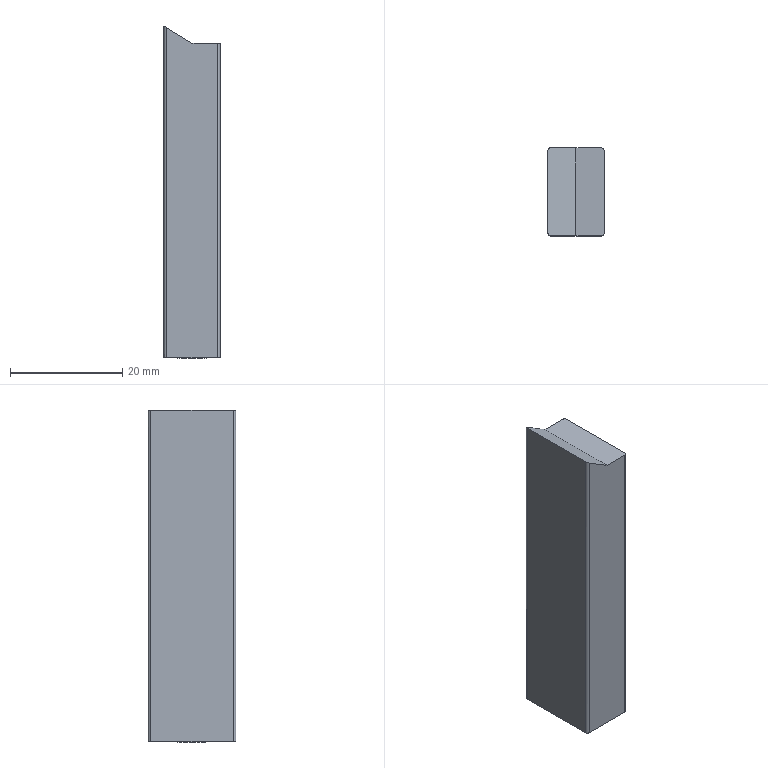Part | STEP file | LUOI GA PHAI TREN | 1 solid | 17 faces | box 10 x 15.6 x 59.05 mm | volume 8567 mm3 | plane 7 | cylinder 6 | cone 4 | commonest cylinder face diameters 1 x4 4.134 x2
STEP:
#1=CARTESIAN_POINT('',(0.,0.,0.));
#2=DIRECTION('',(0.,0.,1.));
#3=DIRECTION('',(1.,0.,0.));
#4=AXIS2_PLACEMENT_3D('',#1,#2,#3);
#5=CARTESIAN_POINT('',(-7.067,7.9,0.5));
#6=VERTEX_POINT('',#5);
#7=CARTESIAN_POINT('',(-7.567,7.9,0.));
#8=VERTEX_POINT('',#7);
#9=CARTESIAN_POINT('',(-7.567,7.9,0.));
#10=DIRECTION('',(-0.7071,0.,-0.7071));
#11=VECTOR('',#10,1.);
#12=LINE('',#9,#11);
#13=CARTESIAN_POINT('',(-5.,7.9,0.));
#14=DIRECTION('',(0.,0.,-1.));
#15=DIRECTION('',(-1.,0.,0.));
#16=AXIS2_PLACEMENT_3D('',#13,#14,#15);
#17=CONICAL_SURFACE('',#16,2.567,0.7854);
#18=CARTESIAN_POINT('',(6.283,0.));
#19=DIRECTION('',(0.,1.));
#20=VECTOR('',#19,1.);
#21=LINE('',#18,#20);
#22=(GEOMETRIC_REPRESENTATION_CONTEXT(2)PARAMETRIC_REPRESENTATION_CONTEXT()REPRESENTATION_CONTEXT('',''));
#23=DEFINITIONAL_REPRESENTATION('',(#21),#22);
#24=PCURVE('',#17,#23);
#25=CARTESIAN_POINT('',(-5.,7.9,0.));
#26=DIRECTION('',(0.,0.,-1.));
#27=DIRECTION('',(-1.,0.,0.));
#28=AXIS2_PLACEMENT_3D('',#25,#26,#27);
#29=CONICAL_SURFACE('',#28,2.567,0.7854);
#30=CARTESIAN_POINT('',(0.,0.));
#31=DIRECTION('',(0.,1.));
#32=VECTOR('',#31,1.);
#33=LINE('',#30,#32);
#34=(GEOMETRIC_REPRESENTATION_CONTEXT(2)PARAMETRIC_REPRESENTATION_CONTEXT()REPRESENTATION_CONTEXT('',''));
#35=DEFINITIONAL_REPRESENTATION('',(#33),#34);
#36=PCURVE('',#29,#35);
#37=SURFACE_CURVE('',#12,(#24,#36),.PCURVE_S1.);
#38=EDGE_CURVE('',#6,#8,#37,.T.);
#39=ORIENTED_EDGE('',*,*,#38,.T.);
#40=CARTESIAN_POINT('',(-2.433,7.9,0.));
#41=VERTEX_POINT('',#40);
#42=CARTESIAN_POINT('',(-5.,7.9,0.));
#43=DIRECTION('',(0.,0.,-1.));
#44=DIRECTION('',(-1.,0.,0.));
#45=AXIS2_PLACEMENT_3D('',#42,#43,#44);
#46=CIRCLE('',#45,2.567);
#47=CARTESIAN_POINT('',(0.,0.));
#48=DIRECTION('',(1.,0.));
#49=VECTOR('',#48,1.);
#50=LINE('',#47,#49);
#51=(GEOMETRIC_REPRESENTATION_CONTEXT(2)PARAMETRIC_REPRESENTATION_CONTEXT()REPRESENTATION_CONTEXT('',''));
#52=DEFINITIONAL_REPRESENTATION('',(#50),#51);
#53=PCURVE('',#17,#52);
#54=CARTESIAN_POINT('',(-5.,7.8,0.));
#55=DIRECTION('',(0.,0.,1.));
#56=DIRECTION('',(1.,0.,0.));
#57=AXIS2_PLACEMENT_3D('',#54,#55,#56);
#58=PLANE('',#57);
#59=CARTESIAN_POINT('',(-2.567,0.1));
#60=CARTESIAN_POINT('',(-2.567,4.546));
#61=CARTESIAN_POINT('',(1.283,2.323));
#62=CARTESIAN_POINT('',(5.134,0.1));
#63=CARTESIAN_POINT('',(1.283,-2.123));
#64=CARTESIAN_POINT('',(-2.567,-4.346));
#65=CARTESIAN_POINT('',(-2.567,0.1));
#66=(BOUNDED_CURVE()B_SPLINE_CURVE(2,(#59,#60,#61,#62,#63,#64,#65),.UNSPECIFIED.,.T.,.F.)B_SPLINE_CURVE_WITH_KNOTS((1,2,2,2,2,1),(-2.094,0.,2.094,4.189,6.283,8.378),.UNSPECIFIED.)CURVE()GEOMETRIC_REPRESENTATION_ITEM()RATIONAL_B_SPLINE_CURVE((1.,0.5,1.,0.5,1.,0.5,1.))REPRESENTATION_ITEM(''));
#67=(GEOMETRIC_REPRESENTATION_CONTEXT(2)PARAMETRIC_REPRESENTATION_CONTEXT()REPRESENTATION_CONTEXT('',''));
#68=DEFINITIONAL_REPRESENTATION('',(#66),#67);
#69=PCURVE('',#58,#68);
#70=SURFACE_CURVE('',#46,(#53,#69),.PCURVE_S1.);
#71=EDGE_CURVE('',#41,#8,#70,.T.);
#72=ORIENTED_EDGE('',*,*,#71,.F.);
#73=CARTESIAN_POINT('',(-2.933,7.9,0.5));
#74=VERTEX_POINT('',#73);
#75=CARTESIAN_POINT('',(-2.433,7.9,0.));
#76=DIRECTION('',(0.7071,0.,-0.7071));
#77=VECTOR('',#76,1.);
#78=LINE('',#75,#77);
#79=CARTESIAN_POINT('',(3.142,0.));
#80=DIRECTION('',(0.,1.));
#81=VECTOR('',#80,1.);
#82=LINE('',#79,#81);
#83=(GEOMETRIC_REPRESENTATION_CONTEXT(2)PARAMETRIC_REPRESENTATION_CONTEXT()REPRESENTATION_CONTEXT('',''));
#84=DEFINITIONAL_REPRESENTATION('',(#82),#83);
#85=PCURVE('',#17,#84);
#86=CARTESIAN_POINT('',(3.142,0.));
#87=DIRECTION('',(0.,1.));
#88=VECTOR('',#87,1.);
#89=LINE('',#86,#88);
#90=(GEOMETRIC_REPRESENTATION_CONTEXT(2)PARAMETRIC_REPRESENTATION_CONTEXT()REPRESENTATION_CONTEXT('',''));
#91=DEFINITIONAL_REPRESENTATION('',(#89),#90);
#92=PCURVE('',#29,#91);
#93=SURFACE_CURVE('',#78,(#85,#92),.PCURVE_S1.);
#94=EDGE_CURVE('',#74,#41,#93,.T.);
#95=ORIENTED_EDGE('',*,*,#94,.F.);
#96=CARTESIAN_POINT('',(-5.,7.9,0.5));
#97=DIRECTION('',(0.,0.,-1.));
#98=DIRECTION('',(1.,0.,0.));
#99=AXIS2_PLACEMENT_3D('',#96,#97,#98);
#100=CIRCLE('',#99,2.067);
#101=CARTESIAN_POINT('',(3.142,-0.5));
#102=DIRECTION('',(1.,0.));
#103=VECTOR('',#102,1.);
#104=LINE('',#101,#103);
#105=(GEOMETRIC_REPRESENTATION_CONTEXT(2)PARAMETRIC_REPRESENTATION_CONTEXT()REPRESENTATION_CONTEXT('',''));
#106=DEFINITIONAL_REPRESENTATION('',(#104),#105);
#107=PCURVE('',#17,#106);
#108=CARTESIAN_POINT('',(-5.,7.9,10.));
#109=DIRECTION('',(0.,0.,-1.));
#110=DIRECTION('',(-1.,0.,0.));
#111=AXIS2_PLACEMENT_3D('',#108,#109,#110);
#112=CYLINDRICAL_SURFACE('',#111,2.067);
#113=CARTESIAN_POINT('',(3.142,9.5));
#114=DIRECTION('',(1.,0.));
#115=VECTOR('',#114,1.);
#116=LINE('',#113,#115);
#117=(GEOMETRIC_REPRESENTATION_CONTEXT(2)PARAMETRIC_REPRESENTATION_CONTEXT()REPRESENTATION_CONTEXT('',''));
#118=DEFINITIONAL_REPRESENTATION('',(#116),#117);
#119=PCURVE('',#112,#118);
#120=SURFACE_CURVE('',#100,(#107,#119),.PCURVE_S1.);
#121=EDGE_CURVE('',#74,#6,#120,.T.);
#122=ORIENTED_EDGE('',*,*,#121,.T.);
#123=EDGE_LOOP('',(#39,#72,#95,#122));
#124=FACE_BOUND('',#123,.F.);
#125=ADVANCED_FACE('',(#124),#17,.F.);
#126=CARTESIAN_POINT('',(-7.067,7.9,20.));
#127=VERTEX_POINT('',#126);
#128=CARTESIAN_POINT('',(-7.067,7.9,10.));
#129=DIRECTION('',(0.,0.,-1.));
#130=VECTOR('',#129,1.);
#131=LINE('',#128,#130);
#132=CARTESIAN_POINT('',(6.283,0.));
#133=DIRECTION('',(0.,1.));
#134=VECTOR('',#133,1.);
#135=LINE('',#132,#134);
#136=(GEOMETRIC_REPRESENTATION_CONTEXT(2)PARAMETRIC_REPRESENTATION_CONTEXT()REPRESENTATION_CONTEXT('',''));
#137=DEFINITIONAL_REPRESENTATION('',(#135),#136);
#138=PCURVE('',#112,#137);
#139=CARTESIAN_POINT('',(-5.,7.9,10.));
#140=DIRECTION('',(0.,0.,-1.));
#141=DIRECTION('',(-1.,0.,0.));
#142=AXIS2_PLACEMENT_3D('',#139,#140,#141);
#143=CYLINDRICAL_SURFACE('',#142,2.067);
#144=CARTESIAN_POINT('',(0.,0.));
#145=DIRECTION('',(0.,1.));
#146=VECTOR('',#145,1.);
#147=LINE('',#144,#146);
#148=(GEOMETRIC_REPRESENTATION_CONTEXT(2)PARAMETRIC_REPRESENTATION_CONTEXT()REPRESENTATION_CONTEXT('',''));
#149=DEFINITIONAL_REPRESENTATION('',(#147),#148);
#150=PCURVE('',#143,#149);
#151=SURFACE_CURVE('',#131,(#138,#150),.PCURVE_S1.);
#152=EDGE_CURVE('',#127,#6,#151,.T.);
#153=ORIENTED_EDGE('',*,*,#152,.T.);
#154=ORIENTED_EDGE('',*,*,#121,.F.);
#155=CARTESIAN_POINT('',(-2.933,7.9,20.));
#156=VERTEX_POINT('',#155);
#157=CARTESIAN_POINT('',(-2.933,7.9,10.));
#158=DIRECTION('',(0.,0.,-1.));
#159=VECTOR('',#158,1.);
#160=LINE('',#157,#159);
#161=CARTESIAN_POINT('',(3.142,0.));
#162=DIRECTION('',(0.,1.));
#163=VECTOR('',#162,1.);
#164=LINE('',#161,#163);
#165=(GEOMETRIC_REPRESENTATION_CONTEXT(2)PARAMETRIC_REPRESENTATION_CONTEXT()REPRESENTATION_CONTEXT('',''));
#166=DEFINITIONAL_REPRESENTATION('',(#164),#165);
#167=PCURVE('',#112,#166);
#168=CARTESIAN_POINT('',(3.142,0.));
#169=DIRECTION('',(0.,1.));
#170=VECTOR('',#169,1.);
#171=LINE('',#168,#170);
#172=(GEOMETRIC_REPRESENTATION_CONTEXT(2)PARAMETRIC_REPRESENTATION_CONTEXT()REPRESENTATION_CONTEXT('',''));
#173=DEFINITIONAL_REPRESENTATION('',(#171),#172);
#174=PCURVE('',#143,#173);
#175=SURFACE_CURVE('',#160,(#167,#174),.PCURVE_S1.);
#176=EDGE_CURVE('',#156,#74,#175,.T.);
#177=ORIENTED_EDGE('',*,*,#176,.F.);
#178=CARTESIAN_POINT('',(-5.,7.9,20.));
#179=DIRECTION('',(0.,0.,-1.));
#180=DIRECTION('',(-1.,0.,0.));
#181=AXIS2_PLACEMENT_3D('',#178,#179,#180);
#182=CIRCLE('',#181,2.067);
#183=CARTESIAN_POINT('',(0.,-10.));
#184=DIRECTION('',(1.,0.));
#185=VECTOR('',#184,1.);
#186=LINE('',#183,#185);
#187=(GEOMETRIC_REPRESENTATION_CONTEXT(2)PARAMETRIC_REPRESENTATION_CONTEXT()REPRESENTATION_CONTEXT('',''));
#188=DEFINITIONAL_REPRESENTATION('',(#186),#187);
#189=PCURVE('',#112,#188);
#190=CARTESIAN_POINT('',(-5.,7.9,20.));
#191=DIRECTION('',(0.,0.,-1.));
#192=DIRECTION('',(-1.,0.,0.));
#193=AXIS2_PLACEMENT_3D('',#190,#191,#192);
#194=CONICAL_SURFACE('',#193,2.067,1.03);
#195=CARTESIAN_POINT('',(0.,0.));
#196=DIRECTION('',(1.,0.));
#197=VECTOR('',#196,1.);
#198=LINE('',#195,#197);
#199=(GEOMETRIC_REPRESENTATION_CONTEXT(2)PARAMETRIC_REPRESENTATION_CONTEXT()REPRESENTATION_CONTEXT('',''));
#200=DEFINITIONAL_REPRESENTATION('',(#198),#199);
#201=PCURVE('',#194,#200);
#202=SURFACE_CURVE('',#182,(#189,#201),.PCURVE_S1.);
#203=EDGE_CURVE('',#156,#127,#202,.T.);
#204=ORIENTED_EDGE('',*,*,#203,.T.);
#205=EDGE_LOOP('',(#153,#154,#177,#204));
#206=FACE_BOUND('',#205,.F.);
#207=ADVANCED_FACE('',(#206),#112,.F.);
#208=ORIENTED_EDGE('',*,*,#203,.F.);
#209=CARTESIAN_POINT('',(-5.,7.9,21.242));
#210=VERTEX_POINT('',#209);
#211=CARTESIAN_POINT('',(-2.933,7.9,20.));
#212=DIRECTION('',(0.8572,0.,-0.515));
#213=VECTOR('',#212,1.);
#214=LINE('',#211,#213);
#215=CARTESIAN_POINT('',(3.142,0.));
#216=DIRECTION('',(0.,1.));
#217=VECTOR('',#216,1.);
#218=LINE('',#215,#217);
#219=(GEOMETRIC_REPRESENTATION_CONTEXT(2)PARAMETRIC_REPRESENTATION_CONTEXT()REPRESENTATION_CONTEXT('',''));
#220=DEFINITIONAL_REPRESENTATION('',(#218),#219);
#221=PCURVE('',#194,#220);
#222=CARTESIAN_POINT('',(-5.,7.9,20.));
#223=DIRECTION('',(0.,0.,-1.));
#224=DIRECTION('',(-1.,0.,0.));
#225=AXIS2_PLACEMENT_3D('',#222,#223,#224);
#226=CONICAL_SURFACE('',#225,2.067,1.03);
#227=CARTESIAN_POINT('',(3.142,0.));
#228=DIRECTION('',(0.,1.));
#229=VECTOR('',#228,1.);
#230=LINE('',#227,#229);
#231=(GEOMETRIC_REPRESENTATION_CONTEXT(2)PARAMETRIC_REPRESENTATION_CONTEXT()REPRESENTATION_CONTEXT('',''));
#232=DEFINITIONAL_REPRESENTATION('',(#230),#231);
#233=PCURVE('',#226,#232);
#234=SURFACE_CURVE('',#214,(#221,#233),.PCURVE_S1.);
#235=EDGE_CURVE('',#210,#156,#234,.T.);
#236=ORIENTED_EDGE('',*,*,#235,.F.);
#237=CARTESIAN_POINT('',(-7.067,7.9,20.));
#238=DIRECTION('',(-0.8572,0.,-0.515));
#239=VECTOR('',#238,1.);
#240=LINE('',#237,#239);
#241=CARTESIAN_POINT('',(6.283,0.));
#242=DIRECTION('',(0.,1.));
#243=VECTOR('',#242,1.);
#244=LINE('',#241,#243);
#245=(GEOMETRIC_REPRESENTATION_CONTEXT(2)PARAMETRIC_REPRESENTATION_CONTEXT()REPRESENTATION_CONTEXT('',''));
#246=DEFINITIONAL_REPRESENTATION('',(#244),#245);
#247=PCURVE('',#194,#246);
#248=CARTESIAN_POINT('',(0.,0.));
#249=DIRECTION('',(0.,1.));
#250=VECTOR('',#249,1.);
#251=LINE('',#248,#250);
#252=(GEOMETRIC_REPRESENTATION_CONTEXT(2)PARAMETRIC_REPRESENTATION_CONTEXT()REPRESENTATION_CONTEXT('',''));
#253=DEFINITIONAL_REPRESENTATION('',(#251),#252);
#254=PCURVE('',#226,#253);
#255=SURFACE_CURVE('',#240,(#247,#254),.PCURVE_S1.);
#256=EDGE_CURVE('',#210,#127,#255,.T.);
#257=ORIENTED_EDGE('',*,*,#256,.T.);
#258=EDGE_LOOP('',(#208,#236,#257));
#259=FACE_BOUND('',#258,.F.);
#260=ADVANCED_FACE('',(#259),#194,.F.);
#261=CARTESIAN_POINT('',(-10.,15.1,59.05));
#262=VERTEX_POINT('',#261);
#263=CARTESIAN_POINT('',(-10.,15.1,0.));
#264=VERTEX_POINT('',#263);
#265=CARTESIAN_POINT('',(-10.,15.1,0.));
#266=DIRECTION('',(0.,0.,-1.));
#267=VECTOR('',#266,1.);
#268=LINE('',#265,#267);
#269=CARTESIAN_POINT('',(-10.,0.,0.));
#270=DIRECTION('',(-1.,0.,0.));
#271=DIRECTION('',(0.,0.,1.));
#272=AXIS2_PLACEMENT_3D('',#269,#270,#271);
#273=PLANE('',#272);
#274=CARTESIAN_POINT('',(0.,15.1));
#275=DIRECTION('',(-1.,0.));
#276=VECTOR('',#275,1.);
#277=LINE('',#274,#276);
#278=(GEOMETRIC_REPRESENTATION_CONTEXT(2)PARAMETRIC_REPRESENTATION_CONTEXT()REPRESENTATION_CONTEXT('',''));
#279=DEFINITIONAL_REPRESENTATION('',(#277),#278);
#280=PCURVE('',#273,#279);
#281=CARTESIAN_POINT('',(-9.5,15.1,0.));
#282=DIRECTION('',(0.,0.,1.));
#283=DIRECTION('',(1.,0.,0.));
#284=AXIS2_PLACEMENT_3D('',#281,#282,#283);
#285=CYLINDRICAL_SURFACE('',#284,0.5);
#286=CARTESIAN_POINT('',(3.142,0.));
#287=DIRECTION('',(0.,-1.));
#288=VECTOR('',#287,1.);
#289=LINE('',#286,#288);
#290=(GEOMETRIC_REPRESENTATION_CONTEXT(2)PARAMETRIC_REPRESENTATION_CONTEXT()REPRESENTATION_CONTEXT('',''));
#291=DEFINITIONAL_REPRESENTATION('',(#289),#290);
#292=PCURVE('',#285,#291);
#293=SURFACE_CURVE('',#268,(#280,#292),.PCURVE_S1.);
#294=EDGE_CURVE('',#262,#264,#293,.T.);
#295=ORIENTED_EDGE('',*,*,#294,.T.);
#296=CARTESIAN_POINT('',(-10.,0.5,0.));
#297=VERTEX_POINT('',#296);
#298=CARTESIAN_POINT('',(-10.,0.,0.));
#299=DIRECTION('',(0.,-1.,0.));
#300=VECTOR('',#299,1.);
#301=LINE('',#298,#300);
#302=CARTESIAN_POINT('',(0.,0.));
#303=DIRECTION('',(0.,-1.));
#304=VECTOR('',#303,1.);
#305=LINE('',#302,#304);
#306=(GEOMETRIC_REPRESENTATION_CONTEXT(2)PARAMETRIC_REPRESENTATION_CONTEXT()REPRESENTATION_CONTEXT('',''));
#307=DEFINITIONAL_REPRESENTATION('',(#305),#306);
#308=PCURVE('',#273,#307);
#309=CARTESIAN_POINT('',(-5.,-7.8));
#310=DIRECTION('',(0.,-1.));
#311=VECTOR('',#310,1.);
#312=LINE('',#309,#311);
#313=(GEOMETRIC_REPRESENTATION_CONTEXT(2)PARAMETRIC_REPRESENTATION_CONTEXT()REPRESENTATION_CONTEXT('',''));
#314=DEFINITIONAL_REPRESENTATION('',(#312),#313);
#315=PCURVE('',#58,#314);
#316=SURFACE_CURVE('',#301,(#308,#315),.PCURVE_S1.);
#317=EDGE_CURVE('',#264,#297,#316,.T.);
#318=ORIENTED_EDGE('',*,*,#317,.T.);
#319=CARTESIAN_POINT('',(-10.,0.5,59.05));
#320=VERTEX_POINT('',#319);
#321=CARTESIAN_POINT('',(-10.,0.5,0.));
#322=DIRECTION('',(0.,0.,1.));
#323=VECTOR('',#322,1.);
#324=LINE('',#321,#323);
#325=CARTESIAN_POINT('',(0.,0.5));
#326=DIRECTION('',(1.,0.));
#327=VECTOR('',#326,1.);
#328=LINE('',#325,#327);
#329=(GEOMETRIC_REPRESENTATION_CONTEXT(2)PARAMETRIC_REPRESENTATION_CONTEXT()REPRESENTATION_CONTEXT('',''));
#330=DEFINITIONAL_REPRESENTATION('',(#328),#329);
#331=PCURVE('',#273,#330);
#332=CARTESIAN_POINT('',(-9.5,0.5,0.));
#333=DIRECTION('',(0.,0.,1.));
#334=DIRECTION('',(1.,0.,0.));
#335=AXIS2_PLACEMENT_3D('',#332,#333,#334);
#336=CYLINDRICAL_SURFACE('',#335,0.5);
#337=CARTESIAN_POINT('',(3.142,0.));
#338=DIRECTION('',(0.,1.));
#339=VECTOR('',#338,1.);
#340=LINE('',#337,#339);
#341=(GEOMETRIC_REPRESENTATION_CONTEXT(2)PARAMETRIC_REPRESENTATION_CONTEXT()REPRESENTATION_CONTEXT('',''));
#342=DEFINITIONAL_REPRESENTATION('',(#340),#341);
#343=PCURVE('',#336,#342);
#344=SURFACE_CURVE('',#324,(#331,#343),.PCURVE_S1.);
#345=EDGE_CURVE('',#297,#320,#344,.T.);
#346=ORIENTED_EDGE('',*,*,#345,.T.);
#347=CARTESIAN_POINT('',(-10.,0.,59.05));
#348=DIRECTION('',(0.,1.,0.));
#349=VECTOR('',#348,1.);
#350=LINE('',#347,#349);
#351=CARTESIAN_POINT('',(59.05,0.));
#352=DIRECTION('',(0.,1.));
#353=VECTOR('',#352,1.);
#354=LINE('',#351,#353);
#355=(GEOMETRIC_REPRESENTATION_CONTEXT(2)PARAMETRIC_REPRESENTATION_CONTEXT()REPRESENTATION_CONTEXT('',''));
#356=DEFINITIONAL_REPRESENTATION('',(#354),#355);
#357=PCURVE('',#273,#356);
#358=CARTESIAN_POINT('',(-10.,0.,59.05));
#359=DIRECTION('',(-0.521,0.,-0.8536));
#360=DIRECTION('',(-0.8536,0.,0.521));
#361=AXIS2_PLACEMENT_3D('',#358,#359,#360);
#362=PLANE('',#361);
#363=CARTESIAN_POINT('',(0.,0.));
#364=DIRECTION('',(0.,1.));
#365=VECTOR('',#364,1.);
#366=LINE('',#363,#365);
#367=(GEOMETRIC_REPRESENTATION_CONTEXT(2)PARAMETRIC_REPRESENTATION_CONTEXT()REPRESENTATION_CONTEXT('',''));
#368=DEFINITIONAL_REPRESENTATION('',(#366),#367);
#369=PCURVE('',#362,#368);
#370=SURFACE_CURVE('',#350,(#357,#369),.PCURVE_S1.);
#371=EDGE_CURVE('',#320,#262,#370,.T.);
#372=ORIENTED_EDGE('',*,*,#371,.T.);
#373=EDGE_LOOP('',(#295,#318,#346,#372));
#374=FACE_BOUND('',#373,.T.);
#375=ADVANCED_FACE('',(#374),#273,.T.);
#376=CARTESIAN_POINT('',(-5.,7.9,0.));
#377=DIRECTION('',(0.,0.,-1.));
#378=DIRECTION('',(-1.,0.,0.));
#379=AXIS2_PLACEMENT_3D('',#376,#377,#378);
#380=CIRCLE('',#379,2.567);
#381=CARTESIAN_POINT('',(-2.567,0.1));
#382=CARTESIAN_POINT('',(-2.567,4.546));
#383=CARTESIAN_POINT('',(1.283,2.323));
#384=CARTESIAN_POINT('',(5.134,0.1));
#385=CARTESIAN_POINT('',(1.283,-2.123));
#386=CARTESIAN_POINT('',(-2.567,-4.346));
#387=CARTESIAN_POINT('',(-2.567,0.1));
#388=(BOUNDED_CURVE()B_SPLINE_CURVE(2,(#381,#382,#383,#384,#385,#386,#387),.UNSPECIFIED.,.T.,.F.)B_SPLINE_CURVE_WITH_KNOTS((1,2,2,2,2,1),(-2.094,0.,2.094,4.189,6.283,8.378),.UNSPECIFIED.)CURVE()GEOMETRIC_REPRESENTATION_ITEM()RATIONAL_B_SPLINE_CURVE((1.,0.5,1.,0.5,1.,0.5,1.))REPRESENTATION_ITEM(''));
#389=(GEOMETRIC_REPRESENTATION_CONTEXT(2)PARAMETRIC_REPRESENTATION_CONTEXT()REPRESENTATION_CONTEXT('',''));
#390=DEFINITIONAL_REPRESENTATION('',(#388),#389);
#391=PCURVE('',#58,#390);
#392=CARTESIAN_POINT('',(0.,0.));
#393=DIRECTION('',(1.,0.));
#394=VECTOR('',#393,1.);
#395=LINE('',#392,#394);
#396=(GEOMETRIC_REPRESENTATION_CONTEXT(2)PARAMETRIC_REPRESENTATION_CONTEXT()REPRESENTATION_CONTEXT('',''));
#397=DEFINITIONAL_REPRESENTATION('',(#395),#396);
#398=PCURVE('',#29,#397);
#399=SURFACE_CURVE('',#380,(#391,#398),.PCURVE_S1.);
#400=EDGE_CURVE('',#8,#41,#399,.T.);
#401=ORIENTED_EDGE('',*,*,#400,.F.);
#402=ORIENTED_EDGE('',*,*,#71,.F.);
#403=EDGE_LOOP('',(#401,#402));
#404=FACE_BOUND('',#403,.T.);
#405=ORIENTED_EDGE('',*,*,#317,.F.);
#406=CARTESIAN_POINT('',(-9.5,15.6,0.));
#407=VERTEX_POINT('',#406);
#408=CARTESIAN_POINT('',(-9.5,15.1,0.));
#409=DIRECTION('',(0.,0.,1.));
#410=DIRECTION('',(1.,0.,0.));
#411=AXIS2_PLACEMENT_3D('',#408,#409,#410);
#412=CIRCLE('',#411,0.5);
#413=CARTESIAN_POINT('',(-4.5,7.3));
#414=DIRECTION('',(1.,0.));
#415=AXIS2_PLACEMENT_2D('',#413,#414);
#416=CIRCLE('',#415,0.5);
#417=(GEOMETRIC_REPRESENTATION_CONTEXT(2)PARAMETRIC_REPRESENTATION_CONTEXT()REPRESENTATION_CONTEXT('',''));
#418=DEFINITIONAL_REPRESENTATION('',(#416),#417);
#419=PCURVE('',#58,#418);
#420=CARTESIAN_POINT('',(0.,0.));
#421=DIRECTION('',(1.,0.));
#422=VECTOR('',#421,1.);
#423=LINE('',#420,#422);
#424=(GEOMETRIC_REPRESENTATION_CONTEXT(2)PARAMETRIC_REPRESENTATION_CONTEXT()REPRESENTATION_CONTEXT('',''));
#425=DEFINITIONAL_REPRESENTATION('',(#423),#424);
#426=PCURVE('',#285,#425);
#427=SURFACE_CURVE('',#412,(#419,#426),.PCURVE_S1.);
#428=EDGE_CURVE('',#407,#264,#427,.T.);
#429=ORIENTED_EDGE('',*,*,#428,.F.);
#430=CARTESIAN_POINT('',(-0.5,15.6,0.));
#431=VERTEX_POINT('',#430);
#432=CARTESIAN_POINT('',(-5.,15.6,0.));
#433=DIRECTION('',(-1.,0.,0.));
#434=VECTOR('',#433,1.);
#435=LINE('',#432,#434);
#436=CARTESIAN_POINT('',(0.,7.8));
#437=DIRECTION('',(-1.,0.));
#438=VECTOR('',#437,1.);
#439=LINE('',#436,#438);
#440=(GEOMETRIC_REPRESENTATION_CONTEXT(2)PARAMETRIC_REPRESENTATION_CONTEXT()REPRESENTATION_CONTEXT('',''));
#441=DEFINITIONAL_REPRESENTATION('',(#439),#440);
#442=PCURVE('',#58,#441);
#443=CARTESIAN_POINT('',(-10.,15.6,0.));
#444=DIRECTION('',(0.,1.,0.));
#445=DIRECTION('',(0.,0.,1.));
#446=AXIS2_PLACEMENT_3D('',#443,#444,#445);
#447=PLANE('',#446);
#448=CARTESIAN_POINT('',(0.,5.));
#449=DIRECTION('',(0.,-1.));
#450=VECTOR('',#449,1.);
#451=LINE('',#448,#450);
#452=(GEOMETRIC_REPRESENTATION_CONTEXT(2)PARAMETRIC_REPRESENTATION_CONTEXT()REPRESENTATION_CONTEXT('',''));
#453=DEFINITIONAL_REPRESENTATION('',(#451),#452);
#454=PCURVE('',#447,#453);
#455=SURFACE_CURVE('',#435,(#442,#454),.PCURVE_S1.);
#456=EDGE_CURVE('',#431,#407,#455,.T.);
#457=ORIENTED_EDGE('',*,*,#456,.F.);
#458=CARTESIAN_POINT('',(0.,15.1,0.));
#459=VERTEX_POINT('',#458);
#460=CARTESIAN_POINT('',(-0.5,15.1,0.));
#461=DIRECTION('',(0.,0.,1.));
#462=DIRECTION('',(1.,0.,0.));
#463=AXIS2_PLACEMENT_3D('',#460,#461,#462);
#464=CIRCLE('',#463,0.5);
#465=CARTESIAN_POINT('',(4.5,7.3));
#466=DIRECTION('',(1.,0.));
#467=AXIS2_PLACEMENT_2D('',#465,#466);
#468=CIRCLE('',#467,0.5);
#469=(GEOMETRIC_REPRESENTATION_CONTEXT(2)PARAMETRIC_REPRESENTATION_CONTEXT()REPRESENTATION_CONTEXT('',''));
#470=DEFINITIONAL_REPRESENTATION('',(#468),#469);
#471=PCURVE('',#58,#470);
#472=CARTESIAN_POINT('',(-0.5,15.1,0.));
#473=DIRECTION('',(0.,0.,1.));
#474=DIRECTION('',(1.,0.,0.));
#475=AXIS2_PLACEMENT_3D('',#472,#473,#474);
#476=CYLINDRICAL_SURFACE('',#475,0.5);
#477=CARTESIAN_POINT('',(0.,0.));
#478=DIRECTION('',(1.,0.));
#479=VECTOR('',#478,1.);
#480=LINE('',#477,#479);
#481=(GEOMETRIC_REPRESENTATION_CONTEXT(2)PARAMETRIC_REPRESENTATION_CONTEXT()REPRESENTATION_CONTEXT('',''));
#482=DEFINITIONAL_REPRESENTATION('',(#480),#481);
#483=PCURVE('',#476,#482);
#484=SURFACE_CURVE('',#464,(#471,#483),.PCURVE_S1.);
#485=EDGE_CURVE('',#459,#431,#484,.T.);
#486=ORIENTED_EDGE('',*,*,#485,.F.);
#487=CARTESIAN_POINT('',(0.,0.5,0.));
#488=VERTEX_POINT('',#487);
#489=CARTESIAN_POINT('',(0.,7.8,0.));
#490=DIRECTION('',(0.,1.,0.));
#491=VECTOR('',#490,1.);
#492=LINE('',#489,#491);
#493=CARTESIAN_POINT('',(5.,0.));
#494=DIRECTION('',(0.,1.));
#495=VECTOR('',#494,1.);
#496=LINE('',#493,#495);
#497=(GEOMETRIC_REPRESENTATION_CONTEXT(2)PARAMETRIC_REPRESENTATION_CONTEXT()REPRESENTATION_CONTEXT('',''));
#498=DEFINITIONAL_REPRESENTATION('',(#496),#497);
#499=PCURVE('',#58,#498);
#500=CARTESIAN_POINT('',(0.,15.6,0.));
#501=DIRECTION('',(1.,0.,0.));
#502=DIRECTION('',(0.,0.,-1.));
#503=AXIS2_PLACEMENT_3D('',#500,#501,#502);
#504=PLANE('',#503);
#505=CARTESIAN_POINT('',(0.,-7.8));
#506=DIRECTION('',(0.,1.));
#507=VECTOR('',#506,1.);
#508=LINE('',#505,#507);
#509=(GEOMETRIC_REPRESENTATION_CONTEXT(2)PARAMETRIC_REPRESENTATION_CONTEXT()REPRESENTATION_CONTEXT('',''));
#510=DEFINITIONAL_REPRESENTATION('',(#508),#509);
#511=PCURVE('',#504,#510);
#512=SURFACE_CURVE('',#492,(#499,#511),.PCURVE_S1.);
#513=EDGE_CURVE('',#488,#459,#512,.T.);
#514=ORIENTED_EDGE('',*,*,#513,.F.);
#515=CARTESIAN_POINT('',(-0.5,0.,0.));
#516=VERTEX_POINT('',#515);
#517=CARTESIAN_POINT('',(-0.5,0.5,0.));
#518=DIRECTION('',(0.,0.,1.));
#519=DIRECTION('',(1.,0.,0.));
#520=AXIS2_PLACEMENT_3D('',#517,#518,#519);
#521=CIRCLE('',#520,0.5);
#522=CARTESIAN_POINT('',(4.5,-7.3));
#523=DIRECTION('',(1.,0.));
#524=AXIS2_PLACEMENT_2D('',#522,#523);
#525=CIRCLE('',#524,0.5);
#526=(GEOMETRIC_REPRESENTATION_CONTEXT(2)PARAMETRIC_REPRESENTATION_CONTEXT()REPRESENTATION_CONTEXT('',''));
#527=DEFINITIONAL_REPRESENTATION('',(#525),#526);
#528=PCURVE('',#58,#527);
#529=CARTESIAN_POINT('',(-0.5,0.5,0.));
#530=DIRECTION('',(0.,0.,1.));
#531=DIRECTION('',(1.,0.,0.));
#532=AXIS2_PLACEMENT_3D('',#529,#530,#531);
#533=CYLINDRICAL_SURFACE('',#532,0.5);
#534=CARTESIAN_POINT('',(0.,0.));
#535=DIRECTION('',(1.,0.));
#536=VECTOR('',#535,1.);
#537=LINE('',#534,#536);
#538=(GEOMETRIC_REPRESENTATION_CONTEXT(2)PARAMETRIC_REPRESENTATION_CONTEXT()REPRESENTATION_CONTEXT('',''));
#539=DEFINITIONAL_REPRESENTATION('',(#537),#538);
#540=PCURVE('',#533,#539);
#541=SURFACE_CURVE('',#521,(#528,#540),.PCURVE_S1.);
#542=EDGE_CURVE('',#516,#488,#541,.T.);
#543=ORIENTED_EDGE('',*,*,#542,.F.);
#544=CARTESIAN_POINT('',(-9.5,0.,0.));
#545=VERTEX_POINT('',#544);
#546=CARTESIAN_POINT('',(-5.,0.,0.));
#547=DIRECTION('',(1.,0.,0.));
#548=VECTOR('',#547,1.);
#549=LINE('',#546,#548);
#550=CARTESIAN_POINT('',(0.,-7.8));
#551=DIRECTION('',(1.,0.));
#552=VECTOR('',#551,1.);
#553=LINE('',#550,#552);
#554=(GEOMETRIC_REPRESENTATION_CONTEXT(2)PARAMETRIC_REPRESENTATION_CONTEXT()REPRESENTATION_CONTEXT('',''));
#555=DEFINITIONAL_REPRESENTATION('',(#553),#554);
#556=PCURVE('',#58,#555);
#557=CARTESIAN_POINT('',(0.,0.,0.));
#558=DIRECTION('',(0.,-1.,0.));
#559=DIRECTION('',(0.,0.,-1.));
#560=AXIS2_PLACEMENT_3D('',#557,#558,#559);
#561=PLANE('',#560);
#562=CARTESIAN_POINT('',(0.,-5.));
#563=DIRECTION('',(0.,1.));
#564=VECTOR('',#563,1.);
#565=LINE('',#562,#564);
#566=(GEOMETRIC_REPRESENTATION_CONTEXT(2)PARAMETRIC_REPRESENTATION_CONTEXT()REPRESENTATION_CONTEXT('',''));
#567=DEFINITIONAL_REPRESENTATION('',(#565),#566);
#568=PCURVE('',#561,#567);
#569=SURFACE_CURVE('',#549,(#556,#568),.PCURVE_S1.);
#570=EDGE_CURVE('',#545,#516,#569,.T.);
#571=ORIENTED_EDGE('',*,*,#570,.F.);
#572=CARTESIAN_POINT('',(-9.5,0.5,0.));
#573=DIRECTION('',(0.,0.,1.));
#574=DIRECTION('',(1.,0.,0.));
#575=AXIS2_PLACEMENT_3D('',#572,#573,#574);
#576=CIRCLE('',#575,0.5);
#577=CARTESIAN_POINT('',(-4.5,-7.3));
#578=DIRECTION('',(1.,0.));
#579=AXIS2_PLACEMENT_2D('',#577,#578);
#580=CIRCLE('',#579,0.5);
#581=(GEOMETRIC_REPRESENTATION_CONTEXT(2)PARAMETRIC_REPRESENTATION_CONTEXT()REPRESENTATION_CONTEXT('',''));
#582=DEFINITIONAL_REPRESENTATION('',(#580),#581);
#583=PCURVE('',#58,#582);
#584=CARTESIAN_POINT('',(0.,0.));
#585=DIRECTION('',(1.,0.));
#586=VECTOR('',#585,1.);
#587=LINE('',#584,#586);
#588=(GEOMETRIC_REPRESENTATION_CONTEXT(2)PARAMETRIC_REPRESENTATION_CONTEXT()REPRESENTATION_CONTEXT('',''));
#589=DEFINITIONAL_REPRESENTATION('',(#587),#588);
#590=PCURVE('',#336,#589);
#591=SURFACE_CURVE('',#576,(#583,#590),.PCURVE_S1.);
#592=EDGE_CURVE('',#297,#545,#591,.T.);
#593=ORIENTED_EDGE('',*,*,#592,.F.);
#594=EDGE_LOOP('',(#405,#429,#457,#486,#514,#543,#571,#593));
#595=FACE_BOUND('',#594,.T.);
#596=ADVANCED_FACE('',(#404,#595),#58,.F.);
#597=ORIENTED_EDGE('',*,*,#428,.T.);
#598=ORIENTED_EDGE('',*,*,#294,.F.);
#599=CARTESIAN_POINT('',(-9.5,15.6,58.745));
#600=VERTEX_POINT('',#599);
#601=CARTESIAN_POINT('',(-10.,15.1,59.05));
#602=CARTESIAN_POINT('',(-10.,15.393,59.05));
#603=CARTESIAN_POINT('',(-9.793,15.6,58.924));
#604=CARTESIAN_POINT('',(-9.5,15.6,58.745));
#605=(BOUNDED_CURVE()B_SPLINE_CURVE(3,(#601,#602,#603,#604),.UNSPECIFIED.,.F.,.F.)B_SPLINE_CURVE_WITH_KNOTS((4,4),(0.,1.571),.PIECEWISE_BEZIER_KNOTS.)CURVE()GEOMETRIC_REPRESENTATION_ITEM()RATIONAL_B_SPLINE_CURVE((1.,0.8047,0.8047,1.))REPRESENTATION_ITEM(''));
#606=CARTESIAN_POINT('',(3.142,59.05));
#607=CARTESIAN_POINT('',(3.12,59.05));
#608=CARTESIAN_POINT('',(3.077,59.05));
#609=CARTESIAN_POINT('',(3.01,59.048));
#610=CARTESIAN_POINT('',(2.942,59.044));
#611=CARTESIAN_POINT('',(2.872,59.039));
#612=CARTESIAN_POINT('',(2.801,59.033));
#613=CARTESIAN_POINT('',(2.729,59.025));
#614=CARTESIAN_POINT('',(2.655,59.015));
#615=CARTESIAN_POINT('',(2.581,59.004));
#616=CARTESIAN_POINT('',(2.507,58.991));
#617=CARTESIAN_POINT('',(2.432,58.976));
#618=CARTESIAN_POINT('',(2.356,58.961));
#619=CARTESIAN_POINT('',(2.281,58.944));
#620=CARTESIAN_POINT('',(2.206,58.926));
#621=CARTESIAN_POINT('',(2.131,58.907));
#622=CARTESIAN_POINT('',(2.057,58.888));
#623=CARTESIAN_POINT('',(1.984,58.867));
#624=CARTESIAN_POINT('',(1.912,58.847));
#625=CARTESIAN_POINT('',(1.841,58.826));
#626=CARTESIAN_POINT('',(1.771,58.805));
#627=CARTESIAN_POINT('',(1.702,58.785));
#628=CARTESIAN_POINT('',(1.636,58.765));
#629=CARTESIAN_POINT('',(1.592,58.751));
#630=CARTESIAN_POINT('',(1.571,58.745));
#631=B_SPLINE_CURVE_WITH_KNOTS('',3,(#606,#607,#608,#609,#610,#611,#612,#613,#614,#615,#616,#617,#618,#619,#620,#621,#622,#623,#624,#625,#626,#627,#628,#629,#630),.UNSPECIFIED.,.F.,.F.,(4,1,1,1,1,1,1,1,1,1,1,1,1,1,1,1,1,1,1,1,1,1,4),(0.,0.0714,0.1428,0.2142,0.2856,0.357,0.4284,0.4998,0.5712,0.6426,0.714,0.7854,0.8568,0.9282,0.9996,1.071,1.142,1.214,1.285,1.357,1.428,1.499,1.571),.QUASI_UNIFORM_KNOTS.);
#632=(GEOMETRIC_REPRESENTATION_CONTEXT(2)PARAMETRIC_REPRESENTATION_CONTEXT()REPRESENTATION_CONTEXT('',''));
#633=DEFINITIONAL_REPRESENTATION('',(#631),#632);
#634=PCURVE('',#285,#633);
#635=CARTESIAN_POINT('',(0.,15.1));
#636=CARTESIAN_POINT('',(0.,15.393));
#637=CARTESIAN_POINT('',(-0.2426,15.6));
#638=CARTESIAN_POINT('',(-0.5858,15.6));
#639=(BOUNDED_CURVE()B_SPLINE_CURVE(3,(#635,#636,#637,#638),.UNSPECIFIED.,.F.,.F.)B_SPLINE_CURVE_WITH_KNOTS((4,4),(0.,1.571),.PIECEWISE_BEZIER_KNOTS.)CURVE()GEOMETRIC_REPRESENTATION_ITEM()RATIONAL_B_SPLINE_CURVE((1.,0.8047,0.8047,1.))REPRESENTATION_ITEM(''));
#640=(GEOMETRIC_REPRESENTATION_CONTEXT(2)PARAMETRIC_REPRESENTATION_CONTEXT()REPRESENTATION_CONTEXT('',''));
#641=DEFINITIONAL_REPRESENTATION('',(#639),#640);
#642=PCURVE('',#362,#641);
#643=SURFACE_CURVE('',#605,(#634,#642),.PCURVE_S1.);
#644=EDGE_CURVE('',#262,#600,#643,.T.);
#645=ORIENTED_EDGE('',*,*,#644,.T.);
#646=CARTESIAN_POINT('',(-9.5,15.6,0.));
#647=DIRECTION('',(0.,0.,-1.));
#648=VECTOR('',#647,1.);
#649=LINE('',#646,#648);
#650=CARTESIAN_POINT('',(1.571,0.));
#651=DIRECTION('',(0.,-1.));
#652=VECTOR('',#651,1.);
#653=LINE('',#650,#652);
#654=(GEOMETRIC_REPRESENTATION_CONTEXT(2)PARAMETRIC_REPRESENTATION_CONTEXT()REPRESENTATION_CONTEXT('',''));
#655=DEFINITIONAL_REPRESENTATION('',(#653),#654);
#656=PCURVE('',#285,#655);
#657=CARTESIAN_POINT('',(0.,0.5));
#658=DIRECTION('',(-1.,0.));
#659=VECTOR('',#658,1.);
#660=LINE('',#657,#659);
#661=(GEOMETRIC_REPRESENTATION_CONTEXT(2)PARAMETRIC_REPRESENTATION_CONTEXT()REPRESENTATION_CONTEXT('',''));
#662=DEFINITIONAL_REPRESENTATION('',(#660),#661);
#663=PCURVE('',#447,#662);
#664=SURFACE_CURVE('',#649,(#656,#663),.PCURVE_S1.);
#665=EDGE_CURVE('',#600,#407,#664,.T.);
#666=ORIENTED_EDGE('',*,*,#665,.T.);
#667=EDGE_LOOP('',(#597,#598,#645,#666));
#668=FACE_BOUND('',#667,.T.);
#669=ADVANCED_FACE('',(#668),#285,.T.);
#670=CARTESIAN_POINT('',(-5.003,0.,56.));
#671=VERTEX_POINT('',#670);
#672=CARTESIAN_POINT('',(-9.5,0.,58.745));
#673=VERTEX_POINT('',#672);
#674=CARTESIAN_POINT('',(-10.,0.,59.05));
#675=DIRECTION('',(-0.8536,0.,0.521));
#676=VECTOR('',#675,1.);
#677=LINE('',#674,#676);
#678=CARTESIAN_POINT('',(0.,0.));
#679=DIRECTION('',(1.,0.));
#680=VECTOR('',#679,1.);
#681=LINE('',#678,#680);
#682=(GEOMETRIC_REPRESENTATION_CONTEXT(2)PARAMETRIC_REPRESENTATION_CONTEXT()REPRESENTATION_CONTEXT('',''));
#683=DEFINITIONAL_REPRESENTATION('',(#681),#682);
#684=PCURVE('',#362,#683);
#685=CARTESIAN_POINT('',(-59.05,-10.));
#686=DIRECTION('',(-0.521,-0.8536));
#687=VECTOR('',#686,1.);
#688=LINE('',#685,#687);
#689=(GEOMETRIC_REPRESENTATION_CONTEXT(2)PARAMETRIC_REPRESENTATION_CONTEXT()REPRESENTATION_CONTEXT('',''));
#690=DEFINITIONAL_REPRESENTATION('',(#688),#689);
#691=PCURVE('',#561,#690);
#692=SURFACE_CURVE('',#677,(#684,#691),.PCURVE_S1.);
#693=EDGE_CURVE('',#671,#673,#692,.T.);
#694=ORIENTED_EDGE('',*,*,#693,.F.);
#695=CARTESIAN_POINT('',(-5.003,15.6,56.));
#696=VERTEX_POINT('',#695);
#697=CARTESIAN_POINT('',(-5.003,0.,56.));
#698=DIRECTION('',(0.,-1.,0.));
#699=VECTOR('',#698,1.);
#700=LINE('',#697,#699);
#701=CARTESIAN_POINT('',(-5.854,0.));
#702=DIRECTION('',(0.,-1.));
#703=VECTOR('',#702,1.);
#704=LINE('',#701,#703);
#705=(GEOMETRIC_REPRESENTATION_CONTEXT(2)PARAMETRIC_REPRESENTATION_CONTEXT()REPRESENTATION_CONTEXT('',''));
#706=DEFINITIONAL_REPRESENTATION('',(#704),#705);
#707=PCURVE('',#362,#706);
#708=CARTESIAN_POINT('',(-5.003,0.,56.));
#709=DIRECTION('',(0.,0.,-1.));
#710=DIRECTION('',(-1.,0.,0.));
#711=AXIS2_PLACEMENT_3D('',#708,#709,#710);
#712=PLANE('',#711);
#713=CARTESIAN_POINT('',(0.,0.));
#714=DIRECTION('',(0.,-1.));
#715=VECTOR('',#714,1.);
#716=LINE('',#713,#715);
#717=(GEOMETRIC_REPRESENTATION_CONTEXT(2)PARAMETRIC_REPRESENTATION_CONTEXT()REPRESENTATION_CONTEXT('',''));
#718=DEFINITIONAL_REPRESENTATION('',(#716),#717);
#719=PCURVE('',#712,#718);
#720=SURFACE_CURVE('',#700,(#707,#719),.PCURVE_S1.);
#721=EDGE_CURVE('',#696,#671,#720,.T.);
#722=ORIENTED_EDGE('',*,*,#721,.F.);
#723=CARTESIAN_POINT('',(-10.,15.6,59.05));
#724=DIRECTION('',(0.8536,0.,-0.521));
#725=VECTOR('',#724,1.);
#726=LINE('',#723,#725);
#727=CARTESIAN_POINT('',(0.,15.6));
#728=DIRECTION('',(-1.,0.));
#729=VECTOR('',#728,1.);
#730=LINE('',#727,#729);
#731=(GEOMETRIC_REPRESENTATION_CONTEXT(2)PARAMETRIC_REPRESENTATION_CONTEXT()REPRESENTATION_CONTEXT('',''));
#732=DEFINITIONAL_REPRESENTATION('',(#730),#731);
#733=PCURVE('',#362,#732);
#734=CARTESIAN_POINT('',(59.05,0.));
#735=DIRECTION('',(-0.521,0.8536));
#736=VECTOR('',#735,1.);
#737=LINE('',#734,#736);
#738=(GEOMETRIC_REPRESENTATION_CONTEXT(2)PARAMETRIC_REPRESENTATION_CONTEXT()REPRESENTATION_CONTEXT('',''));
#739=DEFINITIONAL_REPRESENTATION('',(#737),#738);
#740=PCURVE('',#447,#739);
#741=SURFACE_CURVE('',#726,(#733,#740),.PCURVE_S1.);
#742=EDGE_CURVE('',#600,#696,#741,.T.);
#743=ORIENTED_EDGE('',*,*,#742,.F.);
#744=ORIENTED_EDGE('',*,*,#644,.F.);
#745=ORIENTED_EDGE('',*,*,#371,.F.);
#746=CARTESIAN_POINT('',(-9.5,0.,58.745));
#747=CARTESIAN_POINT('',(-9.793,0.,58.924));
#748=CARTESIAN_POINT('',(-10.,0.2071,59.05));
#749=CARTESIAN_POINT('',(-10.,0.5,59.05));
#750=(BOUNDED_CURVE()B_SPLINE_CURVE(3,(#746,#747,#748,#749),.UNSPECIFIED.,.F.,.F.)B_SPLINE_CURVE_WITH_KNOTS((4,4),(4.712,6.283),.PIECEWISE_BEZIER_KNOTS.)CURVE()GEOMETRIC_REPRESENTATION_ITEM()RATIONAL_B_SPLINE_CURVE((1.,0.8047,0.8047,1.))REPRESENTATION_ITEM(''));
#751=CARTESIAN_POINT('',(-0.5858,0.));
#752=CARTESIAN_POINT('',(-0.2426,0.));
#753=CARTESIAN_POINT('',(0.,0.2071));
#754=CARTESIAN_POINT('',(0.,0.5));
#755=(BOUNDED_CURVE()B_SPLINE_CURVE(3,(#751,#752,#753,#754),.UNSPECIFIED.,.F.,.F.)B_SPLINE_CURVE_WITH_KNOTS((4,4),(4.712,6.283),.PIECEWISE_BEZIER_KNOTS.)CURVE()GEOMETRIC_REPRESENTATION_ITEM()RATIONAL_B_SPLINE_CURVE((1.,0.8047,0.8047,1.))REPRESENTATION_ITEM(''));
#756=(GEOMETRIC_REPRESENTATION_CONTEXT(2)PARAMETRIC_REPRESENTATION_CONTEXT()REPRESENTATION_CONTEXT('',''));
#757=DEFINITIONAL_REPRESENTATION('',(#755),#756);
#758=PCURVE('',#362,#757);
#759=CARTESIAN_POINT('',(4.712,58.745));
#760=CARTESIAN_POINT('',(4.691,58.751));
#761=CARTESIAN_POINT('',(4.648,58.765));
#762=CARTESIAN_POINT('',(4.581,58.785));
#763=CARTESIAN_POINT('',(4.512,58.805));
#764=CARTESIAN_POINT('',(4.443,58.826));
#765=CARTESIAN_POINT('',(4.372,58.847));
#766=CARTESIAN_POINT('',(4.299,58.867));
#767=CARTESIAN_POINT('',(4.226,58.888));
#768=CARTESIAN_POINT('',(4.152,58.907));
#769=CARTESIAN_POINT('',(4.077,58.926));
#770=CARTESIAN_POINT('',(4.002,58.944));
#771=CARTESIAN_POINT('',(3.927,58.961));
#772=CARTESIAN_POINT('',(3.852,58.976));
#773=CARTESIAN_POINT('',(3.777,58.991));
#774=CARTESIAN_POINT('',(3.702,59.004));
#775=CARTESIAN_POINT('',(3.628,59.015));
#776=CARTESIAN_POINT('',(3.555,59.025));
#777=CARTESIAN_POINT('',(3.482,59.033));
#778=CARTESIAN_POINT('',(3.411,59.039));
#779=CARTESIAN_POINT('',(3.342,59.044));
#780=CARTESIAN_POINT('',(3.273,59.048));
#781=CARTESIAN_POINT('',(3.206,59.05));
#782=CARTESIAN_POINT('',(3.163,59.05));
#783=CARTESIAN_POINT('',(3.142,59.05));
#784=B_SPLINE_CURVE_WITH_KNOTS('',3,(#759,#760,#761,#762,#763,#764,#765,#766,#767,#768,#769,#770,#771,#772,#773,#774,#775,#776,#777,#778,#779,#780,#781,#782,#783),.UNSPECIFIED.,.F.,.F.,(4,1,1,1,1,1,1,1,1,1,1,1,1,1,1,1,1,1,1,1,1,1,4),(4.712,4.784,4.855,4.927,4.998,5.069,5.141,5.212,5.284,5.355,5.426,5.498,5.569,5.641,5.712,5.783,5.855,5.926,5.998,6.069,6.14,6.212,6.283),.QUASI_UNIFORM_KNOTS.);
#785=(GEOMETRIC_REPRESENTATION_CONTEXT(2)PARAMETRIC_REPRESENTATION_CONTEXT()REPRESENTATION_CONTEXT('',''));
#786=DEFINITIONAL_REPRESENTATION('',(#784),#785);
#787=PCURVE('',#336,#786);
#788=SURFACE_CURVE('',#750,(#758,#787),.PCURVE_S1.);
#789=EDGE_CURVE('',#673,#320,#788,.T.);
#790=ORIENTED_EDGE('',*,*,#789,.F.);
#791=EDGE_LOOP('',(#694,#722,#743,#744,#745,#790));
#792=FACE_BOUND('',#791,.T.);
#793=ADVANCED_FACE('',(#792),#362,.F.);
#794=ORIENTED_EDGE('',*,*,#592,.T.);
#795=CARTESIAN_POINT('',(-9.5,0.,0.));
#796=DIRECTION('',(0.,0.,1.));
#797=VECTOR('',#796,1.);
#798=LINE('',#795,#797);
#799=CARTESIAN_POINT('',(4.712,0.));
#800=DIRECTION('',(0.,1.));
#801=VECTOR('',#800,1.);
#802=LINE('',#799,#801);
#803=(GEOMETRIC_REPRESENTATION_CONTEXT(2)PARAMETRIC_REPRESENTATION_CONTEXT()REPRESENTATION_CONTEXT('',''));
#804=DEFINITIONAL_REPRESENTATION('',(#802),#803);
#805=PCURVE('',#336,#804);
#806=CARTESIAN_POINT('',(0.,-9.5));
#807=DIRECTION('',(-1.,0.));
#808=VECTOR('',#807,1.);
#809=LINE('',#806,#808);
#810=(GEOMETRIC_REPRESENTATION_CONTEXT(2)PARAMETRIC_REPRESENTATION_CONTEXT()REPRESENTATION_CONTEXT('',''));
#811=DEFINITIONAL_REPRESENTATION('',(#809),#810);
#812=PCURVE('',#561,#811);
#813=SURFACE_CURVE('',#798,(#805,#812),.PCURVE_S1.);
#814=EDGE_CURVE('',#545,#673,#813,.T.);
#815=ORIENTED_EDGE('',*,*,#814,.T.);
#816=ORIENTED_EDGE('',*,*,#789,.T.);
#817=ORIENTED_EDGE('',*,*,#345,.F.);
#818=EDGE_LOOP('',(#794,#815,#816,#817));
#819=FACE_BOUND('',#818,.T.);
#820=ADVANCED_FACE('',(#819),#336,.T.);
#821=ORIENTED_EDGE('',*,*,#400,.F.);
#822=ORIENTED_EDGE('',*,*,#38,.F.);
#823=CARTESIAN_POINT('',(-5.,7.9,0.5));
#824=DIRECTION('',(0.,0.,-1.));
#825=DIRECTION('',(1.,0.,0.));
#826=AXIS2_PLACEMENT_3D('',#823,#824,#825);
#827=CIRCLE('',#826,2.067);
#828=CARTESIAN_POINT('',(-3.142,-0.5));
#829=DIRECTION('',(1.,0.));
#830=VECTOR('',#829,1.);
#831=LINE('',#828,#830);
#832=(GEOMETRIC_REPRESENTATION_CONTEXT(2)PARAMETRIC_REPRESENTATION_CONTEXT()REPRESENTATION_CONTEXT('',''));
#833=DEFINITIONAL_REPRESENTATION('',(#831),#832);
#834=PCURVE('',#29,#833);
#835=CARTESIAN_POINT('',(-3.142,9.5));
#836=DIRECTION('',(1.,0.));
#837=VECTOR('',#836,1.);
#838=LINE('',#835,#837);
#839=(GEOMETRIC_REPRESENTATION_CONTEXT(2)PARAMETRIC_REPRESENTATION_CONTEXT()REPRESENTATION_CONTEXT('',''));
#840=DEFINITIONAL_REPRESENTATION('',(#838),#839);
#841=PCURVE('',#143,#840);
#842=SURFACE_CURVE('',#827,(#834,#841),.PCURVE_S1.);
#843=EDGE_CURVE('',#6,#74,#842,.T.);
#844=ORIENTED_EDGE('',*,*,#843,.T.);
#845=ORIENTED_EDGE('',*,*,#94,.T.);
#846=EDGE_LOOP('',(#821,#822,#844,#845));
#847=FACE_BOUND('',#846,.F.);
#848=ADVANCED_FACE('',(#847),#29,.F.);
#849=CARTESIAN_POINT('',(-0.5,15.6,56.));
#850=VERTEX_POINT('',#849);
#851=CARTESIAN_POINT('',(-0.5,15.6,0.));
#852=DIRECTION('',(0.,0.,-1.));
#853=VECTOR('',#852,1.);
#854=LINE('',#851,#853);
#855=CARTESIAN_POINT('',(0.,9.5));
#856=DIRECTION('',(-1.,0.));
#857=VECTOR('',#856,1.);
#858=LINE('',#855,#857);
#859=(GEOMETRIC_REPRESENTATION_CONTEXT(2)PARAMETRIC_REPRESENTATION_CONTEXT()REPRESENTATION_CONTEXT('',''));
#860=DEFINITIONAL_REPRESENTATION('',(#858),#859);
#861=PCURVE('',#447,#860);
#862=CARTESIAN_POINT('',(1.571,0.));
#863=DIRECTION('',(0.,-1.));
#864=VECTOR('',#863,1.);
#865=LINE('',#862,#864);
#866=(GEOMETRIC_REPRESENTATION_CONTEXT(2)PARAMETRIC_REPRESENTATION_CONTEXT()REPRESENTATION_CONTEXT('',''));
#867=DEFINITIONAL_REPRESENTATION('',(#865),#866);
#868=PCURVE('',#476,#867);
#869=SURFACE_CURVE('',#854,(#861,#868),.PCURVE_S1.);
#870=EDGE_CURVE('',#850,#431,#869,.T.);
#871=ORIENTED_EDGE('',*,*,#870,.T.);
#872=ORIENTED_EDGE('',*,*,#456,.T.);
#873=ORIENTED_EDGE('',*,*,#665,.F.);
#874=ORIENTED_EDGE('',*,*,#742,.T.);
#875=CARTESIAN_POINT('',(-10.,15.6,56.));
#876=DIRECTION('',(1.,0.,0.));
#877=VECTOR('',#876,1.);
#878=LINE('',#875,#877);
#879=CARTESIAN_POINT('',(56.,0.));
#880=DIRECTION('',(0.,1.));
#881=VECTOR('',#880,1.);
#882=LINE('',#879,#881);
#883=(GEOMETRIC_REPRESENTATION_CONTEXT(2)PARAMETRIC_REPRESENTATION_CONTEXT()REPRESENTATION_CONTEXT('',''));
#884=DEFINITIONAL_REPRESENTATION('',(#882),#883);
#885=PCURVE('',#447,#884);
#886=CARTESIAN_POINT('',(4.997,15.6));
#887=DIRECTION('',(-1.,0.));
#888=VECTOR('',#887,1.);
#889=LINE('',#886,#888);
#890=(GEOMETRIC_REPRESENTATION_CONTEXT(2)PARAMETRIC_REPRESENTATION_CONTEXT()REPRESENTATION_CONTEXT('',''));
#891=DEFINITIONAL_REPRESENTATION('',(#889),#890);
#892=PCURVE('',#712,#891);
#893=SURFACE_CURVE('',#878,(#885,#892),.PCURVE_S1.);
#894=EDGE_CURVE('',#696,#850,#893,.T.);
#895=ORIENTED_EDGE('',*,*,#894,.T.);
#896=EDGE_LOOP('',(#871,#872,#873,#874,#895));
#897=FACE_BOUND('',#896,.T.);
#898=ADVANCED_FACE('',(#897),#447,.T.);
#899=CARTESIAN_POINT('',(0.,15.1,56.));
#900=VERTEX_POINT('',#899);
#901=CARTESIAN_POINT('',(0.,15.1,0.));
#902=DIRECTION('',(0.,0.,1.));
#903=VECTOR('',#902,1.);
#904=LINE('',#901,#903);
#905=CARTESIAN_POINT('',(0.,-0.5));
#906=DIRECTION('',(-1.,0.));
#907=VECTOR('',#906,1.);
#908=LINE('',#905,#907);
#909=(GEOMETRIC_REPRESENTATION_CONTEXT(2)PARAMETRIC_REPRESENTATION_CONTEXT()REPRESENTATION_CONTEXT('',''));
#910=DEFINITIONAL_REPRESENTATION('',(#908),#909);
#911=PCURVE('',#504,#910);
#912=CARTESIAN_POINT('',(0.,0.));
#913=DIRECTION('',(0.,1.));
#914=VECTOR('',#913,1.);
#915=LINE('',#912,#914);
#916=(GEOMETRIC_REPRESENTATION_CONTEXT(2)PARAMETRIC_REPRESENTATION_CONTEXT()REPRESENTATION_CONTEXT('',''));
#917=DEFINITIONAL_REPRESENTATION('',(#915),#916);
#918=PCURVE('',#476,#917);
#919=SURFACE_CURVE('',#904,(#911,#918),.PCURVE_S1.);
#920=EDGE_CURVE('',#459,#900,#919,.T.);
#921=ORIENTED_EDGE('',*,*,#920,.T.);
#922=CARTESIAN_POINT('',(0.,0.5,56.));
#923=VERTEX_POINT('',#922);
#924=CARTESIAN_POINT('',(0.,15.6,56.));
#925=DIRECTION('',(0.,-1.,0.));
#926=VECTOR('',#925,1.);
#927=LINE('',#924,#926);
#928=CARTESIAN_POINT('',(-56.,0.));
#929=DIRECTION('',(0.,-1.));
#930=VECTOR('',#929,1.);
#931=LINE('',#928,#930);
#932=(GEOMETRIC_REPRESENTATION_CONTEXT(2)PARAMETRIC_REPRESENTATION_CONTEXT()REPRESENTATION_CONTEXT('',''));
#933=DEFINITIONAL_REPRESENTATION('',(#931),#932);
#934=PCURVE('',#504,#933);
#935=CARTESIAN_POINT('',(-5.003,15.6));
#936=DIRECTION('',(0.,-1.));
#937=VECTOR('',#936,1.);
#938=LINE('',#935,#937);
#939=(GEOMETRIC_REPRESENTATION_CONTEXT(2)PARAMETRIC_REPRESENTATION_CONTEXT()REPRESENTATION_CONTEXT('',''));
#940=DEFINITIONAL_REPRESENTATION('',(#938),#939);
#941=PCURVE('',#712,#940);
#942=SURFACE_CURVE('',#927,(#934,#941),.PCURVE_S1.);
#943=EDGE_CURVE('',#900,#923,#942,.T.);
#944=ORIENTED_EDGE('',*,*,#943,.T.);
#945=CARTESIAN_POINT('',(0.,0.5,0.));
#946=DIRECTION('',(0.,0.,-1.));
#947=VECTOR('',#946,1.);
#948=LINE('',#945,#947);
#949=CARTESIAN_POINT('',(0.,-15.1));
#950=DIRECTION('',(1.,0.));
#951=VECTOR('',#950,1.);
#952=LINE('',#949,#951);
#953=(GEOMETRIC_REPRESENTATION_CONTEXT(2)PARAMETRIC_REPRESENTATION_CONTEXT()REPRESENTATION_CONTEXT('',''));
#954=DEFINITIONAL_REPRESENTATION('',(#952),#953);
#955=PCURVE('',#504,#954);
#956=CARTESIAN_POINT('',(6.283,0.));
#957=DIRECTION('',(0.,-1.));
#958=VECTOR('',#957,1.);
#959=LINE('',#956,#958);
#960=(GEOMETRIC_REPRESENTATION_CONTEXT(2)PARAMETRIC_REPRESENTATION_CONTEXT()REPRESENTATION_CONTEXT('',''));
#961=DEFINITIONAL_REPRESENTATION('',(#959),#960);
#962=PCURVE('',#533,#961);
#963=SURFACE_CURVE('',#948,(#955,#962),.PCURVE_S1.);
#964=EDGE_CURVE('',#923,#488,#963,.T.);
#965=ORIENTED_EDGE('',*,*,#964,.T.);
#966=ORIENTED_EDGE('',*,*,#513,.T.);
#967=EDGE_LOOP('',(#921,#944,#965,#966));
#968=FACE_BOUND('',#967,.T.);
#969=ADVANCED_FACE('',(#968),#504,.T.);
#970=CARTESIAN_POINT('',(-0.5,0.,56.));
#971=VERTEX_POINT('',#970);
#972=CARTESIAN_POINT('',(0.,0.,56.));
#973=DIRECTION('',(-1.,0.,0.));
#974=VECTOR('',#973,1.);
#975=LINE('',#972,#974);
#976=CARTESIAN_POINT('',(-56.,0.));
#977=DIRECTION('',(0.,-1.));
#978=VECTOR('',#977,1.);
#979=LINE('',#976,#978);
#980=(GEOMETRIC_REPRESENTATION_CONTEXT(2)PARAMETRIC_REPRESENTATION_CONTEXT()REPRESENTATION_CONTEXT('',''));
#981=DEFINITIONAL_REPRESENTATION('',(#979),#980);
#982=PCURVE('',#561,#981);
#983=CARTESIAN_POINT('',(-5.003,0.));
#984=DIRECTION('',(1.,0.));
#985=VECTOR('',#984,1.);
#986=LINE('',#983,#985);
#987=(GEOMETRIC_REPRESENTATION_CONTEXT(2)PARAMETRIC_REPRESENTATION_CONTEXT()REPRESENTATION_CONTEXT('',''));
#988=DEFINITIONAL_REPRESENTATION('',(#986),#987);
#989=PCURVE('',#712,#988);
#990=SURFACE_CURVE('',#975,(#982,#989),.PCURVE_S1.);
#991=EDGE_CURVE('',#971,#671,#990,.T.);
#992=ORIENTED_EDGE('',*,*,#991,.T.);
#993=ORIENTED_EDGE('',*,*,#693,.T.);
#994=ORIENTED_EDGE('',*,*,#814,.F.);
#995=ORIENTED_EDGE('',*,*,#570,.T.);
#996=CARTESIAN_POINT('',(-0.5,0.,0.));
#997=DIRECTION('',(0.,0.,1.));
#998=VECTOR('',#997,1.);
#999=LINE('',#996,#998);
#1000=CARTESIAN_POINT('',(0.,-0.5));
#1001=DIRECTION('',(-1.,0.));
#1002=VECTOR('',#1001,1.);
#1003=LINE('',#1000,#1002);
#1004=(GEOMETRIC_REPRESENTATION_CONTEXT(2)PARAMETRIC_REPRESENTATION_CONTEXT()REPRESENTATION_CONTEXT('',''));
#1005=DEFINITIONAL_REPRESENTATION('',(#1003),#1004);
#1006=PCURVE('',#561,#1005);
#1007=CARTESIAN_POINT('',(4.712,0.));
#1008=DIRECTION('',(0.,1.));
#1009=VECTOR('',#1008,1.);
#1010=LINE('',#1007,#1009);
#1011=(GEOMETRIC_REPRESENTATION_CONTEXT(2)PARAMETRIC_REPRESENTATION_CONTEXT()REPRESENTATION_CONTEXT('',''));
#1012=DEFINITIONAL_REPRESENTATION('',(#1010),#1011);
#1013=PCURVE('',#533,#1012);
#1014=SURFACE_CURVE('',#999,(#1006,#1013),.PCURVE_S1.);
#1015=EDGE_CURVE('',#516,#971,#1014,.T.);
#1016=ORIENTED_EDGE('',*,*,#1015,.T.);
#1017=EDGE_LOOP('',(#992,#993,#994,#995,#1016));
#1018=FACE_BOUND('',#1017,.T.);
#1019=ADVANCED_FACE('',(#1018),#561,.T.);
#1020=ORIENTED_EDGE('',*,*,#943,.F.);
#1021=CARTESIAN_POINT('',(-0.5,15.1,56.));
#1022=DIRECTION('',(0.,0.,-1.));
#1023=DIRECTION('',(1.,0.,0.));
#1024=AXIS2_PLACEMENT_3D('',#1021,#1022,#1023);
#1025=CIRCLE('',#1024,0.5);
#1026=CARTESIAN_POINT('',(-4.503,15.1));
#1027=DIRECTION('',(-1.,0.));
#1028=AXIS2_PLACEMENT_2D('',#1026,#1027);
#1029=CIRCLE('',#1028,0.5);
#1030=(GEOMETRIC_REPRESENTATION_CONTEXT(2)PARAMETRIC_REPRESENTATION_CONTEXT()REPRESENTATION_CONTEXT('',''));
#1031=DEFINITIONAL_REPRESENTATION('',(#1029),#1030);
#1032=PCURVE('',#712,#1031);
#1033=CARTESIAN_POINT('',(6.283,56.));
#1034=DIRECTION('',(-1.,0.));
#1035=VECTOR('',#1034,1.);
#1036=LINE('',#1033,#1035);
#1037=(GEOMETRIC_REPRESENTATION_CONTEXT(2)PARAMETRIC_REPRESENTATION_CONTEXT()REPRESENTATION_CONTEXT('',''));
#1038=DEFINITIONAL_REPRESENTATION('',(#1036),#1037);
#1039=PCURVE('',#476,#1038);
#1040=SURFACE_CURVE('',#1025,(#1032,#1039),.PCURVE_S1.);
#1041=EDGE_CURVE('',#850,#900,#1040,.T.);
#1042=ORIENTED_EDGE('',*,*,#1041,.F.);
#1043=ORIENTED_EDGE('',*,*,#894,.F.);
#1044=ORIENTED_EDGE('',*,*,#721,.T.);
#1045=ORIENTED_EDGE('',*,*,#991,.F.);
#1046=CARTESIAN_POINT('',(-0.5,0.5,56.));
#1047=DIRECTION('',(0.,0.,-1.));
#1048=DIRECTION('',(1.,0.,0.));
#1049=AXIS2_PLACEMENT_3D('',#1046,#1047,#1048);
#1050=CIRCLE('',#1049,0.5);
#1051=CARTESIAN_POINT('',(-4.503,0.5));
#1052=DIRECTION('',(-1.,0.));
#1053=AXIS2_PLACEMENT_2D('',#1051,#1052);
#1054=CIRCLE('',#1053,0.5);
#1055=(GEOMETRIC_REPRESENTATION_CONTEXT(2)PARAMETRIC_REPRESENTATION_CONTEXT()REPRESENTATION_CONTEXT('',''));
#1056=DEFINITIONAL_REPRESENTATION('',(#1054),#1055);
#1057=PCURVE('',#712,#1056);
#1058=CARTESIAN_POINT('',(6.283,56.));
#1059=DIRECTION('',(-1.,0.));
#1060=VECTOR('',#1059,1.);
#1061=LINE('',#1058,#1060);
#1062=(GEOMETRIC_REPRESENTATION_CONTEXT(2)PARAMETRIC_REPRESENTATION_CONTEXT()REPRESENTATION_CONTEXT('',''));
#1063=DEFINITIONAL_REPRESENTATION('',(#1061),#1062);
#1064=PCURVE('',#533,#1063);
#1065=SURFACE_CURVE('',#1050,(#1057,#1064),.PCURVE_S1.);
#1066=EDGE_CURVE('',#923,#971,#1065,.T.);
#1067=ORIENTED_EDGE('',*,*,#1066,.F.);
#1068=EDGE_LOOP('',(#1020,#1042,#1043,#1044,#1045,#1067));
#1069=FACE_BOUND('',#1068,.T.);
#1070=ADVANCED_FACE('',(#1069),#712,.F.);
#1071=ORIENTED_EDGE('',*,*,#843,.F.);
#1072=ORIENTED_EDGE('',*,*,#152,.F.);
#1073=CARTESIAN_POINT('',(-5.,7.9,20.));
#1074=DIRECTION('',(0.,0.,-1.));
#1075=DIRECTION('',(-1.,0.,0.));
#1076=AXIS2_PLACEMENT_3D('',#1073,#1074,#1075);
#1077=CIRCLE('',#1076,2.067);
#1078=CARTESIAN_POINT('',(0.,-10.));
#1079=DIRECTION('',(1.,0.));
#1080=VECTOR('',#1079,1.);
#1081=LINE('',#1078,#1080);
#1082=(GEOMETRIC_REPRESENTATION_CONTEXT(2)PARAMETRIC_REPRESENTATION_CONTEXT()REPRESENTATION_CONTEXT('',''));
#1083=DEFINITIONAL_REPRESENTATION('',(#1081),#1082);
#1084=PCURVE('',#143,#1083);
#1085=CARTESIAN_POINT('',(0.,0.));
#1086=DIRECTION('',(1.,0.));
#1087=VECTOR('',#1086,1.);
#1088=LINE('',#1085,#1087);
#1089=(GEOMETRIC_REPRESENTATION_CONTEXT(2)PARAMETRIC_REPRESENTATION_CONTEXT()REPRESENTATION_CONTEXT('',''));
#1090=DEFINITIONAL_REPRESENTATION('',(#1088),#1089);
#1091=PCURVE('',#226,#1090);
#1092=SURFACE_CURVE('',#1077,(#1084,#1091),.PCURVE_S1.);
#1093=EDGE_CURVE('',#127,#156,#1092,.T.);
#1094=ORIENTED_EDGE('',*,*,#1093,.T.);
#1095=ORIENTED_EDGE('',*,*,#176,.T.);
#1096=EDGE_LOOP('',(#1071,#1072,#1094,#1095));
#1097=FACE_BOUND('',#1096,.F.);
#1098=ADVANCED_FACE('',(#1097),#143,.F.);
#1099=ORIENTED_EDGE('',*,*,#485,.T.);
#1100=ORIENTED_EDGE('',*,*,#870,.F.);
#1101=ORIENTED_EDGE('',*,*,#1041,.T.);
#1102=ORIENTED_EDGE('',*,*,#920,.F.);
#1103=EDGE_LOOP('',(#1099,#1100,#1101,#1102));
#1104=FACE_BOUND('',#1103,.T.);
#1105=ADVANCED_FACE('',(#1104),#476,.T.);
#1106=ORIENTED_EDGE('',*,*,#542,.T.);
#1107=ORIENTED_EDGE('',*,*,#964,.F.);
#1108=ORIENTED_EDGE('',*,*,#1066,.T.);
#1109=ORIENTED_EDGE('',*,*,#1015,.F.);
#1110=EDGE_LOOP('',(#1106,#1107,#1108,#1109));
#1111=FACE_BOUND('',#1110,.T.);
#1112=ADVANCED_FACE('',(#1111),#533,.T.);
#1113=ORIENTED_EDGE('',*,*,#1093,.F.);
#1114=ORIENTED_EDGE('',*,*,#256,.F.);
#1115=ORIENTED_EDGE('',*,*,#235,.T.);
#1116=EDGE_LOOP('',(#1113,#1114,#1115));
#1117=FACE_BOUND('',#1116,.F.);
#1118=ADVANCED_FACE('',(#1117),#226,.F.);
#1119=CLOSED_SHELL('',(#125,#207,#260,#375,#596,#669,#793,#820,#848,#898,#969,#1019,#1070,#1098,#1105,#1112,#1118));
#1120=MANIFOLD_SOLID_BREP('',#1119);
#1121=(LENGTH_UNIT()NAMED_UNIT(*)SI_UNIT(.MILLI.,.METRE.));
#1122=UNCERTAINTY_MEASURE_WITH_UNIT(LENGTH_MEASURE(0.0000001),#1121,'','');
#1123=(NAMED_UNIT(*)PLANE_ANGLE_UNIT()SI_UNIT($,.RADIAN.));
#1124=(NAMED_UNIT(*)SI_UNIT($,.STERADIAN.)SOLID_ANGLE_UNIT());
#1125=(GEOMETRIC_REPRESENTATION_CONTEXT(3)GLOBAL_UNCERTAINTY_ASSIGNED_CONTEXT((#1122))GLOBAL_UNIT_ASSIGNED_CONTEXT((#1121,#1123,#1124))REPRESENTATION_CONTEXT('',''));
#1126=ADVANCED_BREP_SHAPE_REPRESENTATION('',(#4,#1120),#1125);